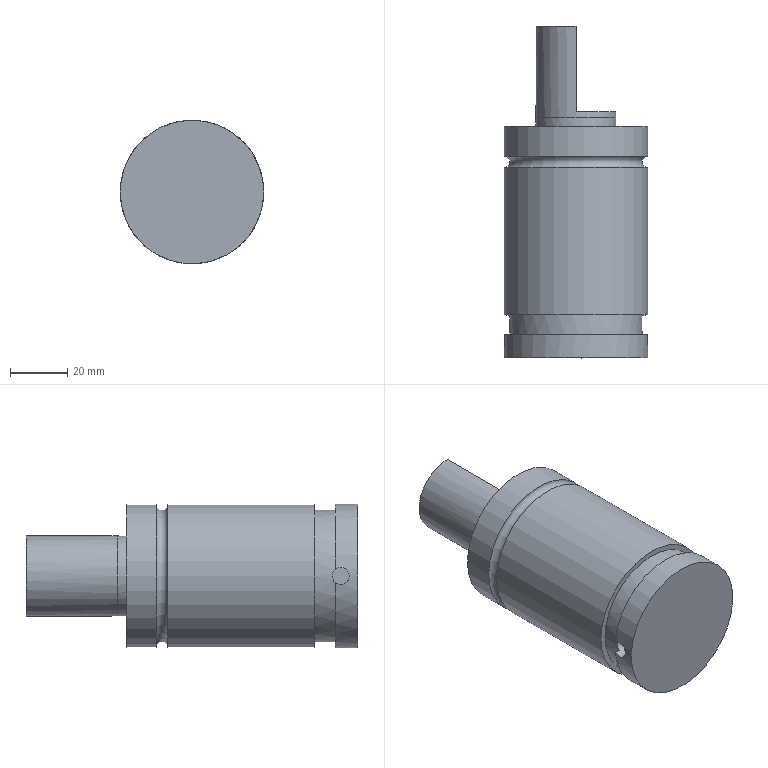Part | NX | features MAIN_BODY 2 | 1 solid | 16 faces | box 50.2 x 116 x 50.2 mm | volume 169326 mm3 | plane 8 | cylinder 7 | torus 1 | commonest cylinder face diameters 50.2 x3 6 x1 27.98 x1 28 x1 46.2 x1
STEP:
#1=CARTESIAN_POINT('',(360.1,544.,150.));
#2=VERTEX_POINT('',#1);
#3=CARTESIAN_POINT('',(335.,544.,150.));
#4=DIRECTION('',(0.,-1.,0.));
#5=DIRECTION('',(1.,0.,0.));
#6=AXIS2_PLACEMENT_3D('',#3,#4,#5);
#7=CIRCLE('',#6,25.1);
#8=EDGE_CURVE('',#2,#2,#7,.F.);
#9=ORIENTED_EDGE('',*,*,#8,.T.);
#10=EDGE_LOOP('',(#9));
#11=FACE_BOUND('',#10,.T.);
#12=CARTESIAN_POINT('',(360.1,595.5,150.));
#13=VERTEX_POINT('',#12);
#14=CARTESIAN_POINT('',(335.,595.5,150.));
#15=DIRECTION('',(0.,-1.,0.));
#16=DIRECTION('',(1.,0.,0.));
#17=AXIS2_PLACEMENT_3D('',#14,#15,#16);
#18=CIRCLE('',#17,25.1);
#19=EDGE_CURVE('',#13,#13,#18,.T.);
#20=ORIENTED_EDGE('',*,*,#19,.T.);
#21=EDGE_LOOP('',(#20));
#22=FACE_BOUND('',#21,.T.);
#23=CARTESIAN_POINT('',(335.,610.,150.));
#24=DIRECTION('',(0.,-1.,0.));
#25=DIRECTION('',(1.,0.,0.));
#26=AXIS2_PLACEMENT_3D('',#23,#24,#25);
#27=CYLINDRICAL_SURFACE('',#26,25.1);
#28=ADVANCED_FACE('',(#11,#22),#27,.T.);
#29=CARTESIAN_POINT('',(309.9,610.,150.));
#30=VERTEX_POINT('',#29);
#31=CARTESIAN_POINT('',(335.,610.,150.));
#32=DIRECTION('',(0.,1.,0.));
#33=DIRECTION('',(-1.,0.,0.));
#34=AXIS2_PLACEMENT_3D('',#31,#32,#33);
#35=CIRCLE('',#34,25.1);
#36=EDGE_CURVE('',#30,#30,#35,.T.);
#37=ORIENTED_EDGE('',*,*,#36,.T.);
#38=EDGE_LOOP('',(#37));
#39=FACE_BOUND('',#38,.T.);
#40=CARTESIAN_POINT('',(321.,610.,150.));
#41=VERTEX_POINT('',#40);
#42=CARTESIAN_POINT('',(335.,610.,150.));
#43=DIRECTION('',(0.,1.,0.));
#44=DIRECTION('',(-1.,0.,0.));
#45=AXIS2_PLACEMENT_3D('',#42,#43,#44);
#46=CIRCLE('',#45,14.);
#47=EDGE_CURVE('',#41,#41,#46,.T.);
#48=ORIENTED_EDGE('',*,*,#47,.F.);
#49=EDGE_LOOP('',(#48));
#50=FACE_BOUND('',#49,.T.);
#51=CARTESIAN_POINT('',(335.,610.,150.));
#52=DIRECTION('',(0.,1.,0.));
#53=DIRECTION('',(-1.,0.,0.));
#54=AXIS2_PLACEMENT_3D('',#51,#52,#53);
#55=PLANE('',#54);
#56=ADVANCED_FACE('',(#39,#50),#55,.T.);
#57=CARTESIAN_POINT('',(360.1,599.5,150.));
#58=VERTEX_POINT('',#57);
#59=CARTESIAN_POINT('',(335.,599.5,150.));
#60=DIRECTION('',(0.,-1.,0.));
#61=DIRECTION('',(1.,0.,0.));
#62=AXIS2_PLACEMENT_3D('',#59,#60,#61);
#63=CIRCLE('',#62,25.1);
#64=EDGE_CURVE('',#58,#58,#63,.F.);
#65=ORIENTED_EDGE('',*,*,#64,.T.);
#66=EDGE_LOOP('',(#65));
#67=FACE_BOUND('',#66,.T.);
#68=ORIENTED_EDGE('',*,*,#36,.F.);
#69=EDGE_LOOP('',(#68));
#70=FACE_BOUND('',#69,.T.);
#71=CARTESIAN_POINT('',(335.,610.,150.));
#72=DIRECTION('',(0.,-1.,0.));
#73=DIRECTION('',(1.,0.,0.));
#74=AXIS2_PLACEMENT_3D('',#71,#72,#73);
#75=CYLINDRICAL_SURFACE('',#74,25.1);
#76=ADVANCED_FACE('',(#67,#70),#75,.T.);
#77=CARTESIAN_POINT('',(325.121,613.,140.094));
#78=VERTEX_POINT('',#77);
#79=CARTESIAN_POINT('',(319.485,613.,149.978));
#80=CARTESIAN_POINT('',(324.045,613.,139.014));
#81=CARTESIAN_POINT('',(335.022,613.,134.485));
#82=CARTESIAN_POINT('',(345.986,613.,139.045));
#83=CARTESIAN_POINT('',(350.515,613.,150.022));
#84=CARTESIAN_POINT('',(345.955,613.,160.986));
#85=CARTESIAN_POINT('',(334.978,613.,165.515));
#86=CARTESIAN_POINT('',(324.014,613.,160.955));
#87=CARTESIAN_POINT('',(319.485,613.,149.978));
#88=CARTESIAN_POINT('',(324.045,613.,139.014));
#89=CARTESIAN_POINT('',(335.022,613.,134.485));
#90=B_SPLINE_CURVE_WITH_KNOTS('',3,(#79,#80,#81,#82,#83,#84,#85,#86,#87,#88,#89),.UNSPECIFIED.,.T.,.F.,(1,1,1,1,1,1,1,1,1,1,1,1,1,1,1),(-0.2498,-0.1248,0.0002218,0.1252,0.2502,0.3752,0.5002,0.6252,0.7502,0.8752,1.,1.125,1.25,1.375,1.5),.UNSPECIFIED.);
#91=EDGE_CURVE('',#78,#78,#90,.F.);
#92=ORIENTED_EDGE('',*,*,#91,.F.);
#93=EDGE_LOOP('',(#92));
#94=FACE_BOUND('',#93,.T.);
#95=ORIENTED_EDGE('',*,*,#47,.T.);
#96=EDGE_LOOP('',(#95));
#97=FACE_BOUND('',#96,.T.);
#98=CARTESIAN_POINT('',(335.,613.,150.));
#99=DIRECTION('',(0.,-1.,0.));
#100=DIRECTION('',(1.,0.,0.));
#101=AXIS2_PLACEMENT_3D('',#98,#99,#100);
#102=CYLINDRICAL_SURFACE('',#101,14.);
#103=ADVANCED_FACE('',(#94,#97),#102,.T.);
#104=ORIENTED_EDGE('',*,*,#64,.F.);
#105=EDGE_LOOP('',(#104));
#106=FACE_BOUND('',#105,.T.);
#107=ORIENTED_EDGE('',*,*,#19,.F.);
#108=EDGE_LOOP('',(#107));
#109=FACE_BOUND('',#108,.T.);
#110=CARTESIAN_POINT('',(335.,597.5,150.));
#111=DIRECTION('',(0.,-1.,0.));
#112=DIRECTION('',(1.,0.,0.));
#113=AXIS2_PLACEMENT_3D('',#110,#111,#112);
#114=TOROIDAL_SURFACE('',#113,25.1,2.);
#115=ADVANCED_FACE('',(#106,#109),#114,.F.);
#116=CARTESIAN_POINT('',(311.9,544.,150.));
#117=VERTEX_POINT('',#116);
#118=CARTESIAN_POINT('',(335.,544.,150.));
#119=DIRECTION('',(0.,1.,0.));
#120=DIRECTION('',(-1.,0.,0.));
#121=AXIS2_PLACEMENT_3D('',#118,#119,#120);
#122=CIRCLE('',#121,23.1);
#123=EDGE_CURVE('',#117,#117,#122,.T.);
#124=ORIENTED_EDGE('',*,*,#123,.T.);
#125=EDGE_LOOP('',(#124));
#126=FACE_BOUND('',#125,.T.);
#127=ORIENTED_EDGE('',*,*,#8,.F.);
#128=EDGE_LOOP('',(#127));
#129=FACE_BOUND('',#128,.T.);
#130=CARTESIAN_POINT('',(335.,544.,150.));
#131=DIRECTION('',(0.,-1.,0.));
#132=DIRECTION('',(1.,0.,0.));
#133=AXIS2_PLACEMENT_3D('',#130,#131,#132);
#134=PLANE('',#133);
#135=ADVANCED_FACE('',(#126,#129),#134,.T.);
#136=CARTESIAN_POINT('',(312.008,537.,152.236));
#137=VERTEX_POINT('',#136);
#138=CARTESIAN_POINT('',(312.008,537.,147.764));
#139=VERTEX_POINT('',#138);
#140=CARTESIAN_POINT('',(335.,537.,150.));
#141=DIRECTION('',(0.,1.,0.));
#142=DIRECTION('',(-1.,0.,0.));
#143=AXIS2_PLACEMENT_3D('',#140,#141,#142);
#144=CIRCLE('',#143,23.1);
#145=EDGE_CURVE('',#137,#139,#144,.T.);
#146=ORIENTED_EDGE('',*,*,#145,.F.);
#147=CARTESIAN_POINT('',(310.,537.,152.236));
#148=VERTEX_POINT('',#147);
#149=CARTESIAN_POINT('',(317.4,537.,152.236));
#150=DIRECTION('',(-1.,0.,0.));
#151=VECTOR('',#150,1000.);
#152=LINE('',#149,#151);
#153=EDGE_CURVE('',#137,#148,#152,.T.);
#154=ORIENTED_EDGE('',*,*,#153,.T.);
#155=CARTESIAN_POINT('',(310.,537.,147.764));
#156=VERTEX_POINT('',#155);
#157=CARTESIAN_POINT('',(335.,537.,150.));
#158=DIRECTION('',(0.,-1.,0.));
#159=DIRECTION('',(1.,0.,0.));
#160=AXIS2_PLACEMENT_3D('',#157,#158,#159);
#161=CIRCLE('',#160,25.1);
#162=EDGE_CURVE('',#156,#148,#161,.T.);
#163=ORIENTED_EDGE('',*,*,#162,.F.);
#164=CARTESIAN_POINT('',(317.4,537.,147.764));
#165=DIRECTION('',(-1.,0.,0.));
#166=VECTOR('',#165,1000.);
#167=LINE('',#164,#166);
#168=EDGE_CURVE('',#156,#139,#167,.F.);
#169=ORIENTED_EDGE('',*,*,#168,.T.);
#170=EDGE_LOOP('',(#146,#154,#163,#169));
#171=FACE_BOUND('',#170,.T.);
#172=CARTESIAN_POINT('',(335.,537.,150.));
#173=DIRECTION('',(0.,-1.,0.));
#174=DIRECTION('',(1.,0.,0.));
#175=AXIS2_PLACEMENT_3D('',#172,#173,#174);
#176=PLANE('',#175);
#177=ADVANCED_FACE('',(#171),#176,.F.);
#178=CARTESIAN_POINT('',(312.008,537.,152.236));
#179=CARTESIAN_POINT('',(311.953,537.632,151.671));
#180=CARTESIAN_POINT('',(311.847,538.368,150.));
#181=CARTESIAN_POINT('',(311.953,537.632,148.329));
#182=CARTESIAN_POINT('',(312.008,537.,147.764));
#183=B_SPLINE_CURVE_WITH_KNOTS('',3,(#178,#179,#180,#181,#182),.UNSPECIFIED.,.F.,.F.,(4,1,4),(0.,0.002514,0.005028),.UNSPECIFIED.);
#184=EDGE_CURVE('',#137,#139,#183,.T.);
#185=ORIENTED_EDGE('',*,*,#184,.F.);
#186=ORIENTED_EDGE('',*,*,#145,.T.);
#187=EDGE_LOOP('',(#185,#186));
#188=FACE_BOUND('',#187,.T.);
#189=ORIENTED_EDGE('',*,*,#123,.F.);
#190=EDGE_LOOP('',(#189));
#191=FACE_BOUND('',#190,.T.);
#192=CARTESIAN_POINT('',(335.,537.,150.));
#193=DIRECTION('',(0.,1.,0.));
#194=DIRECTION('',(-1.,0.,0.));
#195=AXIS2_PLACEMENT_3D('',#192,#193,#194);
#196=CYLINDRICAL_SURFACE('',#195,23.1);
#197=ADVANCED_FACE('',(#188,#191),#196,.T.);
#198=CARTESIAN_POINT('',(309.9,529.,150.));
#199=VERTEX_POINT('',#198);
#200=CARTESIAN_POINT('',(335.,529.,150.));
#201=DIRECTION('',(0.,1.,0.));
#202=DIRECTION('',(-1.,0.,0.));
#203=AXIS2_PLACEMENT_3D('',#200,#201,#202);
#204=CIRCLE('',#203,25.1);
#205=EDGE_CURVE('',#199,#199,#204,.T.);
#206=ORIENTED_EDGE('',*,*,#205,.F.);
#207=EDGE_LOOP('',(#206));
#208=FACE_BOUND('',#207,.T.);
#209=CARTESIAN_POINT('',(335.,529.,150.));
#210=DIRECTION('',(0.,1.,0.));
#211=DIRECTION('',(-1.,0.,0.));
#212=AXIS2_PLACEMENT_3D('',#209,#210,#211);
#213=PLANE('',#212);
#214=ADVANCED_FACE('',(#208),#213,.F.);
#215=ORIENTED_EDGE('',*,*,#162,.T.);
#216=CARTESIAN_POINT('',(310.,537.,152.236));
#217=CARTESIAN_POINT('',(310.069,536.135,153.009));
#218=CARTESIAN_POINT('',(310.115,533.482,153.404));
#219=CARTESIAN_POINT('',(309.792,531.26,150.004));
#220=CARTESIAN_POINT('',(310.115,533.479,146.595));
#221=CARTESIAN_POINT('',(310.069,536.135,146.991));
#222=CARTESIAN_POINT('',(310.,537.,147.764));
#223=B_SPLINE_CURVE_WITH_KNOTS('',3,(#216,#217,#218,#219,#220,#221,#222),.UNSPECIFIED.,.F.,.F.,(4,1,1,1,4),(0.,0.003437,0.006873,0.01031,0.01375),.UNSPECIFIED.);
#224=EDGE_CURVE('',#148,#156,#223,.T.);
#225=ORIENTED_EDGE('',*,*,#224,.T.);
#226=EDGE_LOOP('',(#215,#225));
#227=FACE_BOUND('',#226,.T.);
#228=ORIENTED_EDGE('',*,*,#205,.T.);
#229=EDGE_LOOP('',(#228));
#230=FACE_BOUND('',#229,.T.);
#231=CARTESIAN_POINT('',(335.,583.,150.));
#232=DIRECTION('',(0.,-1.,0.));
#233=DIRECTION('',(1.,0.,0.));
#234=AXIS2_PLACEMENT_3D('',#231,#232,#233);
#235=CYLINDRICAL_SURFACE('',#234,25.1);
#236=ADVANCED_FACE('',(#227,#230),#235,.T.);
#237=ORIENTED_EDGE('',*,*,#184,.T.);
#238=ORIENTED_EDGE('',*,*,#168,.F.);
#239=ORIENTED_EDGE('',*,*,#224,.F.);
#240=ORIENTED_EDGE('',*,*,#153,.F.);
#241=EDGE_LOOP('',(#237,#238,#239,#240));
#242=FACE_BOUND('',#241,.T.);
#243=CARTESIAN_POINT('',(317.4,535.,153.));
#244=VERTEX_POINT('',#243);
#245=CARTESIAN_POINT('',(317.4,535.,150.));
#246=DIRECTION('',(-1.,0.,0.));
#247=DIRECTION('',(0.,0.,1.));
#248=AXIS2_PLACEMENT_3D('',#245,#246,#247);
#249=CIRCLE('',#248,3.);
#250=EDGE_CURVE('',#244,#244,#249,.T.);
#251=ORIENTED_EDGE('',*,*,#250,.F.);
#252=EDGE_LOOP('',(#251));
#253=FACE_BOUND('',#252,.T.);
#254=CARTESIAN_POINT('',(317.4,535.,150.));
#255=DIRECTION('',(-1.,0.,0.));
#256=DIRECTION('',(0.,-1.,0.));
#257=AXIS2_PLACEMENT_3D('',#254,#255,#256);
#258=CYLINDRICAL_SURFACE('',#257,3.);
#259=ADVANCED_FACE('',(#242,#253),#258,.F.);
#260=ORIENTED_EDGE('',*,*,#250,.T.);
#261=EDGE_LOOP('',(#260));
#262=FACE_BOUND('',#261,.T.);
#263=CARTESIAN_POINT('',(317.4,535.,150.));
#264=DIRECTION('',(-1.,0.,0.));
#265=DIRECTION('',(0.,-1.,0.));
#266=AXIS2_PLACEMENT_3D('',#263,#264,#265);
#267=PLANE('',#266);
#268=ADVANCED_FACE('',(#262),#267,.T.);
#269=ORIENTED_EDGE('',*,*,#91,.T.);
#270=EDGE_LOOP('',(#269));
#271=FACE_BOUND('',#270,.T.);
#272=CARTESIAN_POINT('',(335.,645.,163.99));
#273=VERTEX_POINT('',#272);
#274=CARTESIAN_POINT('',(335.,615.,163.99));
#275=VERTEX_POINT('',#274);
#276=CARTESIAN_POINT('',(335.,632.,163.99));
#277=DIRECTION('',(0.,-1.,0.));
#278=VECTOR('',#277,1000.);
#279=LINE('',#276,#278);
#280=EDGE_CURVE('',#273,#275,#279,.T.);
#281=ORIENTED_EDGE('',*,*,#280,.F.);
#282=CARTESIAN_POINT('',(335.,645.,136.01));
#283=VERTEX_POINT('',#282);
#284=CARTESIAN_POINT('',(335.,645.,150.));
#285=DIRECTION('',(0.,1.,0.));
#286=DIRECTION('',(0.,0.,1.));
#287=AXIS2_PLACEMENT_3D('',#284,#285,#286);
#288=CIRCLE('',#287,13.99);
#289=EDGE_CURVE('',#283,#273,#288,.T.);
#290=ORIENTED_EDGE('',*,*,#289,.F.);
#291=CARTESIAN_POINT('',(335.,615.,136.01));
#292=VERTEX_POINT('',#291);
#293=CARTESIAN_POINT('',(335.,617.,136.01));
#294=DIRECTION('',(0.,-1.,0.));
#295=VECTOR('',#294,1000.);
#296=LINE('',#293,#295);
#297=EDGE_CURVE('',#292,#283,#296,.F.);
#298=ORIENTED_EDGE('',*,*,#297,.F.);
#299=CARTESIAN_POINT('',(335.,615.,150.));
#300=DIRECTION('',(0.,-1.,0.));
#301=DIRECTION('',(0.,0.,-1.));
#302=AXIS2_PLACEMENT_3D('',#299,#300,#301);
#303=CIRCLE('',#302,13.99);
#304=EDGE_CURVE('',#292,#275,#303,.T.);
#305=ORIENTED_EDGE('',*,*,#304,.T.);
#306=EDGE_LOOP('',(#281,#290,#298,#305));
#307=FACE_BOUND('',#306,.T.);
#308=CARTESIAN_POINT('',(335.,632.,150.));
#309=DIRECTION('',(0.,-1.,0.));
#310=DIRECTION('',(1.,0.,0.));
#311=AXIS2_PLACEMENT_3D('',#308,#309,#310);
#312=CYLINDRICAL_SURFACE('',#311,13.99);
#313=ADVANCED_FACE('',(#271,#307),#312,.T.);
#314=ORIENTED_EDGE('',*,*,#289,.T.);
#315=CARTESIAN_POINT('',(335.,645.,150.));
#316=DIRECTION('',(0.,0.,-1.));
#317=VECTOR('',#316,1000.);
#318=LINE('',#315,#317);
#319=EDGE_CURVE('',#273,#283,#318,.T.);
#320=ORIENTED_EDGE('',*,*,#319,.T.);
#321=EDGE_LOOP('',(#314,#320));
#322=FACE_BOUND('',#321,.T.);
#323=CARTESIAN_POINT('',(335.,645.,150.));
#324=DIRECTION('',(0.,1.,0.));
#325=DIRECTION('',(-1.,0.,0.));
#326=AXIS2_PLACEMENT_3D('',#323,#324,#325);
#327=PLANE('',#326);
#328=ADVANCED_FACE('',(#322),#327,.T.);
#329=CARTESIAN_POINT('',(335.,615.,332.203));
#330=DIRECTION('',(0.,0.,-1.));
#331=VECTOR('',#330,1000.);
#332=LINE('',#329,#331);
#333=EDGE_CURVE('',#275,#292,#332,.T.);
#334=ORIENTED_EDGE('',*,*,#333,.F.);
#335=ORIENTED_EDGE('',*,*,#304,.F.);
#336=EDGE_LOOP('',(#334,#335));
#337=FACE_BOUND('',#336,.T.);
#338=CARTESIAN_POINT('',(335.,615.,332.203));
#339=DIRECTION('',(0.,-1.,0.));
#340=DIRECTION('',(1.,0.,0.));
#341=AXIS2_PLACEMENT_3D('',#338,#339,#340);
#342=PLANE('',#341);
#343=ADVANCED_FACE('',(#337),#342,.F.);
#344=ORIENTED_EDGE('',*,*,#280,.T.);
#345=ORIENTED_EDGE('',*,*,#333,.T.);
#346=ORIENTED_EDGE('',*,*,#297,.T.);
#347=ORIENTED_EDGE('',*,*,#319,.F.);
#348=EDGE_LOOP('',(#344,#345,#346,#347));
#349=FACE_BOUND('',#348,.T.);
#350=CARTESIAN_POINT('',(335.,617.,332.203));
#351=DIRECTION('',(1.,0.,0.));
#352=DIRECTION('',(0.,0.,-1.));
#353=AXIS2_PLACEMENT_3D('',#350,#351,#352);
#354=PLANE('',#353);
#355=ADVANCED_FACE('',(#349),#354,.T.);
#356=CLOSED_SHELL('',(#28,#56,#76,#103,#115,#135,#177,#197,#214,#236,#259,#268,#313,#328,#343,#355));
#357=MANIFOLD_SOLID_BREP('',#356);
#358=(LENGTH_UNIT()NAMED_UNIT(*)SI_UNIT(.MILLI.,.METRE.));
#359=UNCERTAINTY_MEASURE_WITH_UNIT(LENGTH_MEASURE(0.0508),#358,'','');
#360=(NAMED_UNIT(*)PLANE_ANGLE_UNIT()SI_UNIT($,.RADIAN.));
#361=(NAMED_UNIT(*)SI_UNIT($,.STERADIAN.)SOLID_ANGLE_UNIT());
#362=(GEOMETRIC_REPRESENTATION_CONTEXT(3)GLOBAL_UNCERTAINTY_ASSIGNED_CONTEXT((#359))GLOBAL_UNIT_ASSIGNED_CONTEXT((#358,#360,#361))REPRESENTATION_CONTEXT('',''));
#363=ADVANCED_BREP_SHAPE_REPRESENTATION('',(#357),#362);